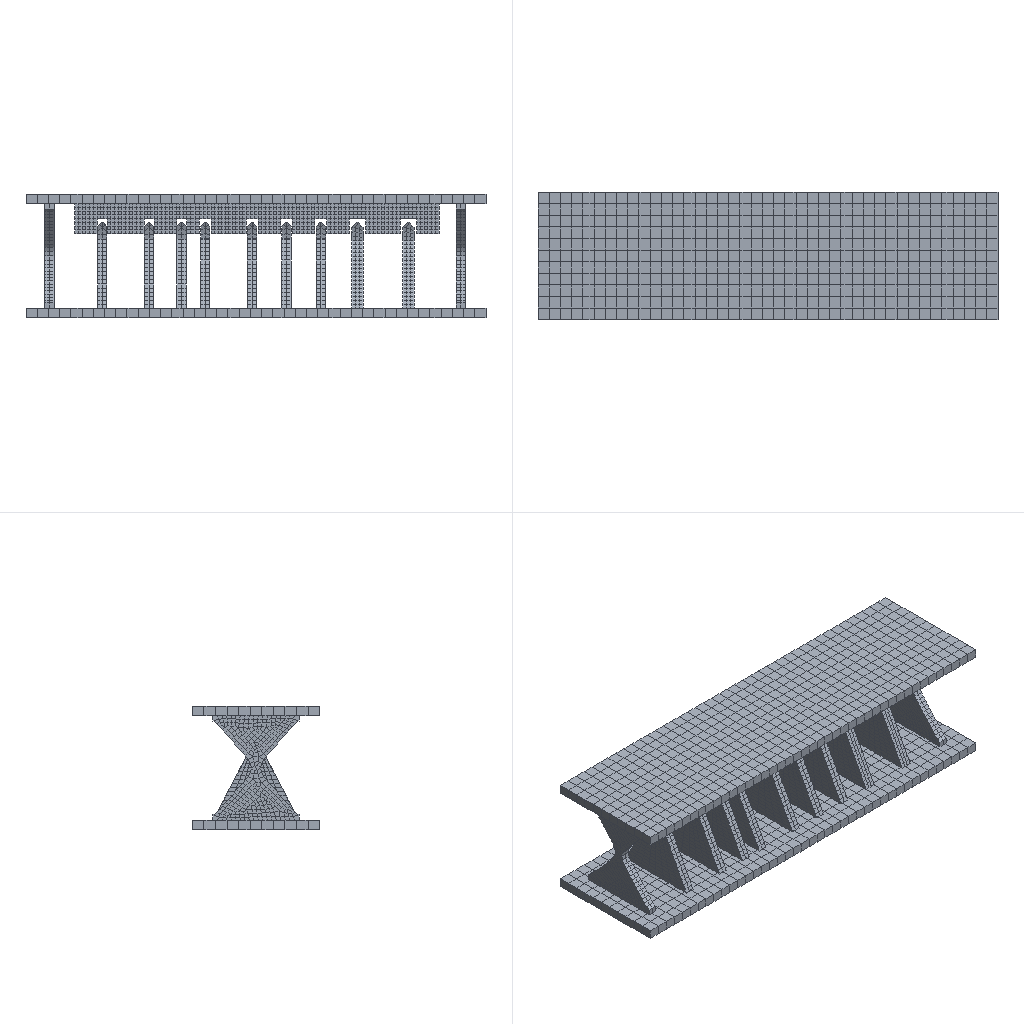Simulation study | abaqus
Set-up summary:
category,name,step,type,value,unit,region
solver,abaqus,,Abaqus/CAE 2024
units,mm-N-s-tonne (MPa),,inferred,E=206000 density=7.85e-09
analysis,Step-1,,static,nlgeom=True; time_period=80
analysis,Step-1,,static,nlgeom=True; time_period=1
mesh,deck-1.inp,,nodes,14009
mesh,deck-1.inp,,elements,8164
element_type,C3D8R,,,8164,,deck-1.inp
mesh,deck-2.inp,,nodes,14009
mesh,deck-2.inp,,elements,8164
element_type,C3D8R,,,8164,,deck-2.inp
material,q235,,E,206000
material,q235,,nu,0.3
material,q235,,density,7.85e-09
material,q235,,yield,220
material,q235,,behaviors,plastic
section,q235,,solid section,,,_PickedSet5
section,q235,,solid section,,,Set-1
section,q235,,solid section,,,Set-1
section,q235,,solid section,,,Set-1
section,q235,,solid section,,,_PickedSet10
section,q235,,solid section,,,Set-1
section,q235,,solid section,,,_PickedSet5
section,q235,,solid section,,,Set-1
section,q235,,solid section,,,Set-1
section,q235,,solid section,,,Set-1
section,q235,,solid section,,,_PickedSet10
section,q235,,solid section,,,Set-1
bc,BC-4,initial,encastre,[dofs=ENCASTRE n=2],,_PickedSet121
bc,BC-3,Step-1,displacement,10 [dofs=x n=2],,_PickedSet120
bc,BC-3,Step-1,fixed,"[dofs=rx,ry,rz,y,z n=10]",,_PickedSet120
contact,Constraint-2,initial,tie,,,s_Surf-26 / m_Surf-12
contact,Constraint-3,initial,tie,,,s_Surf-27 / m_Surf-13
contact,Int-1,initial,contact pair surface to surface,interaction=IntProp-1; friction=0.3; behavior=hard,,s_Surf-28 / m_Surf-30
contact,Constraint-2,initial,tie,,,s_Surf-26 / m_Surf-12
contact,Constraint-3,initial,tie,,,s_Surf-27 / m_Surf-13
contact,Int-1,initial,contact pair surface to surface,interaction=IntProp-1; friction=0.3; behavior=hard,,s_Surf-28 / m_Surf-30
constraint,coupling,,,4
Results summary:
result,odb.job_status,,,JOB_STATUS_COMPLETED_SUCCESSFULLY,"consistent, unstated (Abaqus has no unit system)"
result,steps[0].procedure,Step-1,,*STATIC,"consistent, unstated (Abaqus has no unit system)"
result,steps[0].time_period,Step-1,,1,"consistent, unstated (Abaqus has no unit system)"
result,steps[0].n_frames,Step-1,,21,"consistent, unstated (Abaqus has no unit system)"
result,steps[0].last_frame.id,Step-1,,20,"consistent, unstated (Abaqus has no unit system)"
result,steps[0].last_frame.value,Step-1,,1,"consistent, unstated (Abaqus has no unit system)"
result,steps[0].last_frame.description,Step-1,,Increment     20: Step Time =    1.000,"consistent, unstated (Abaqus has no unit system)"
result,steps[0].completed,Step-1,,True,"consistent, unstated (Abaqus has no unit system)"
result,steps[0].max_U_magnitude,Step-1,,11.178,"consistent, unstated (Abaqus has no unit system)"
result,steps[0].max_S_mises,Step-1,,227.991,"consistent, unstated (Abaqus has no unit system)"
result,steps[0].RF_sum[1],Step-1,,2880.81,"consistent, unstated (Abaqus has no unit system)"
result,steps[0].RF_sum[2],Step-1,,1.785,"consistent, unstated (Abaqus has no unit system)"
result,steps[0].RF_sum[3],Step-1,,-255.141,"consistent, unstated (Abaqus has no unit system)"